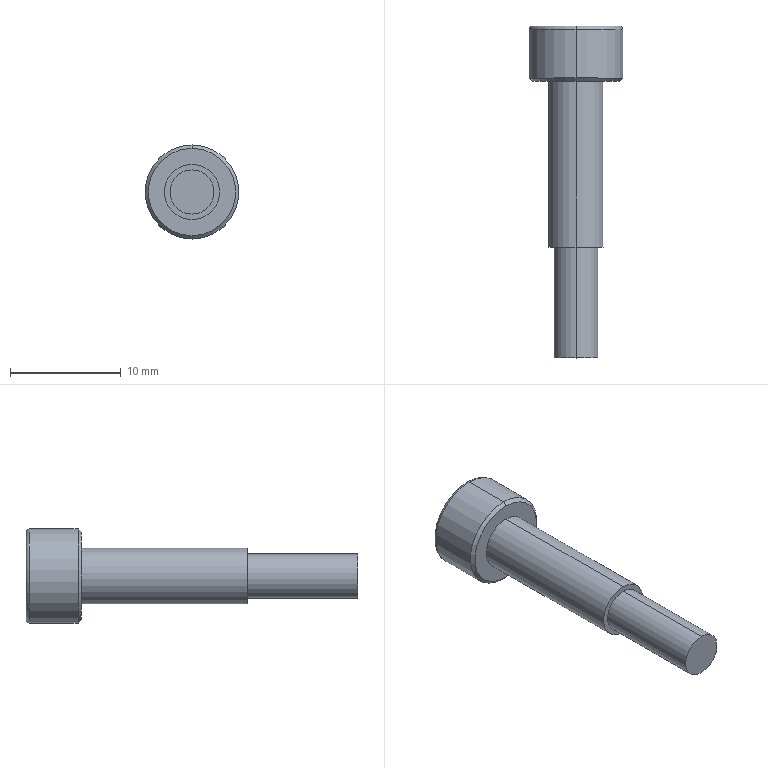Part | STEP file | 1 solid | 51 faces | box 8.5 x 30 x 8.5 mm | volume 658.629 mm3 | cylinder 24 | plane 11 | torus 8 | sphere 6 | cone 2 | commonest cylinder face diameters 0.6 x18 4 x2 5 x2 8.5 x2